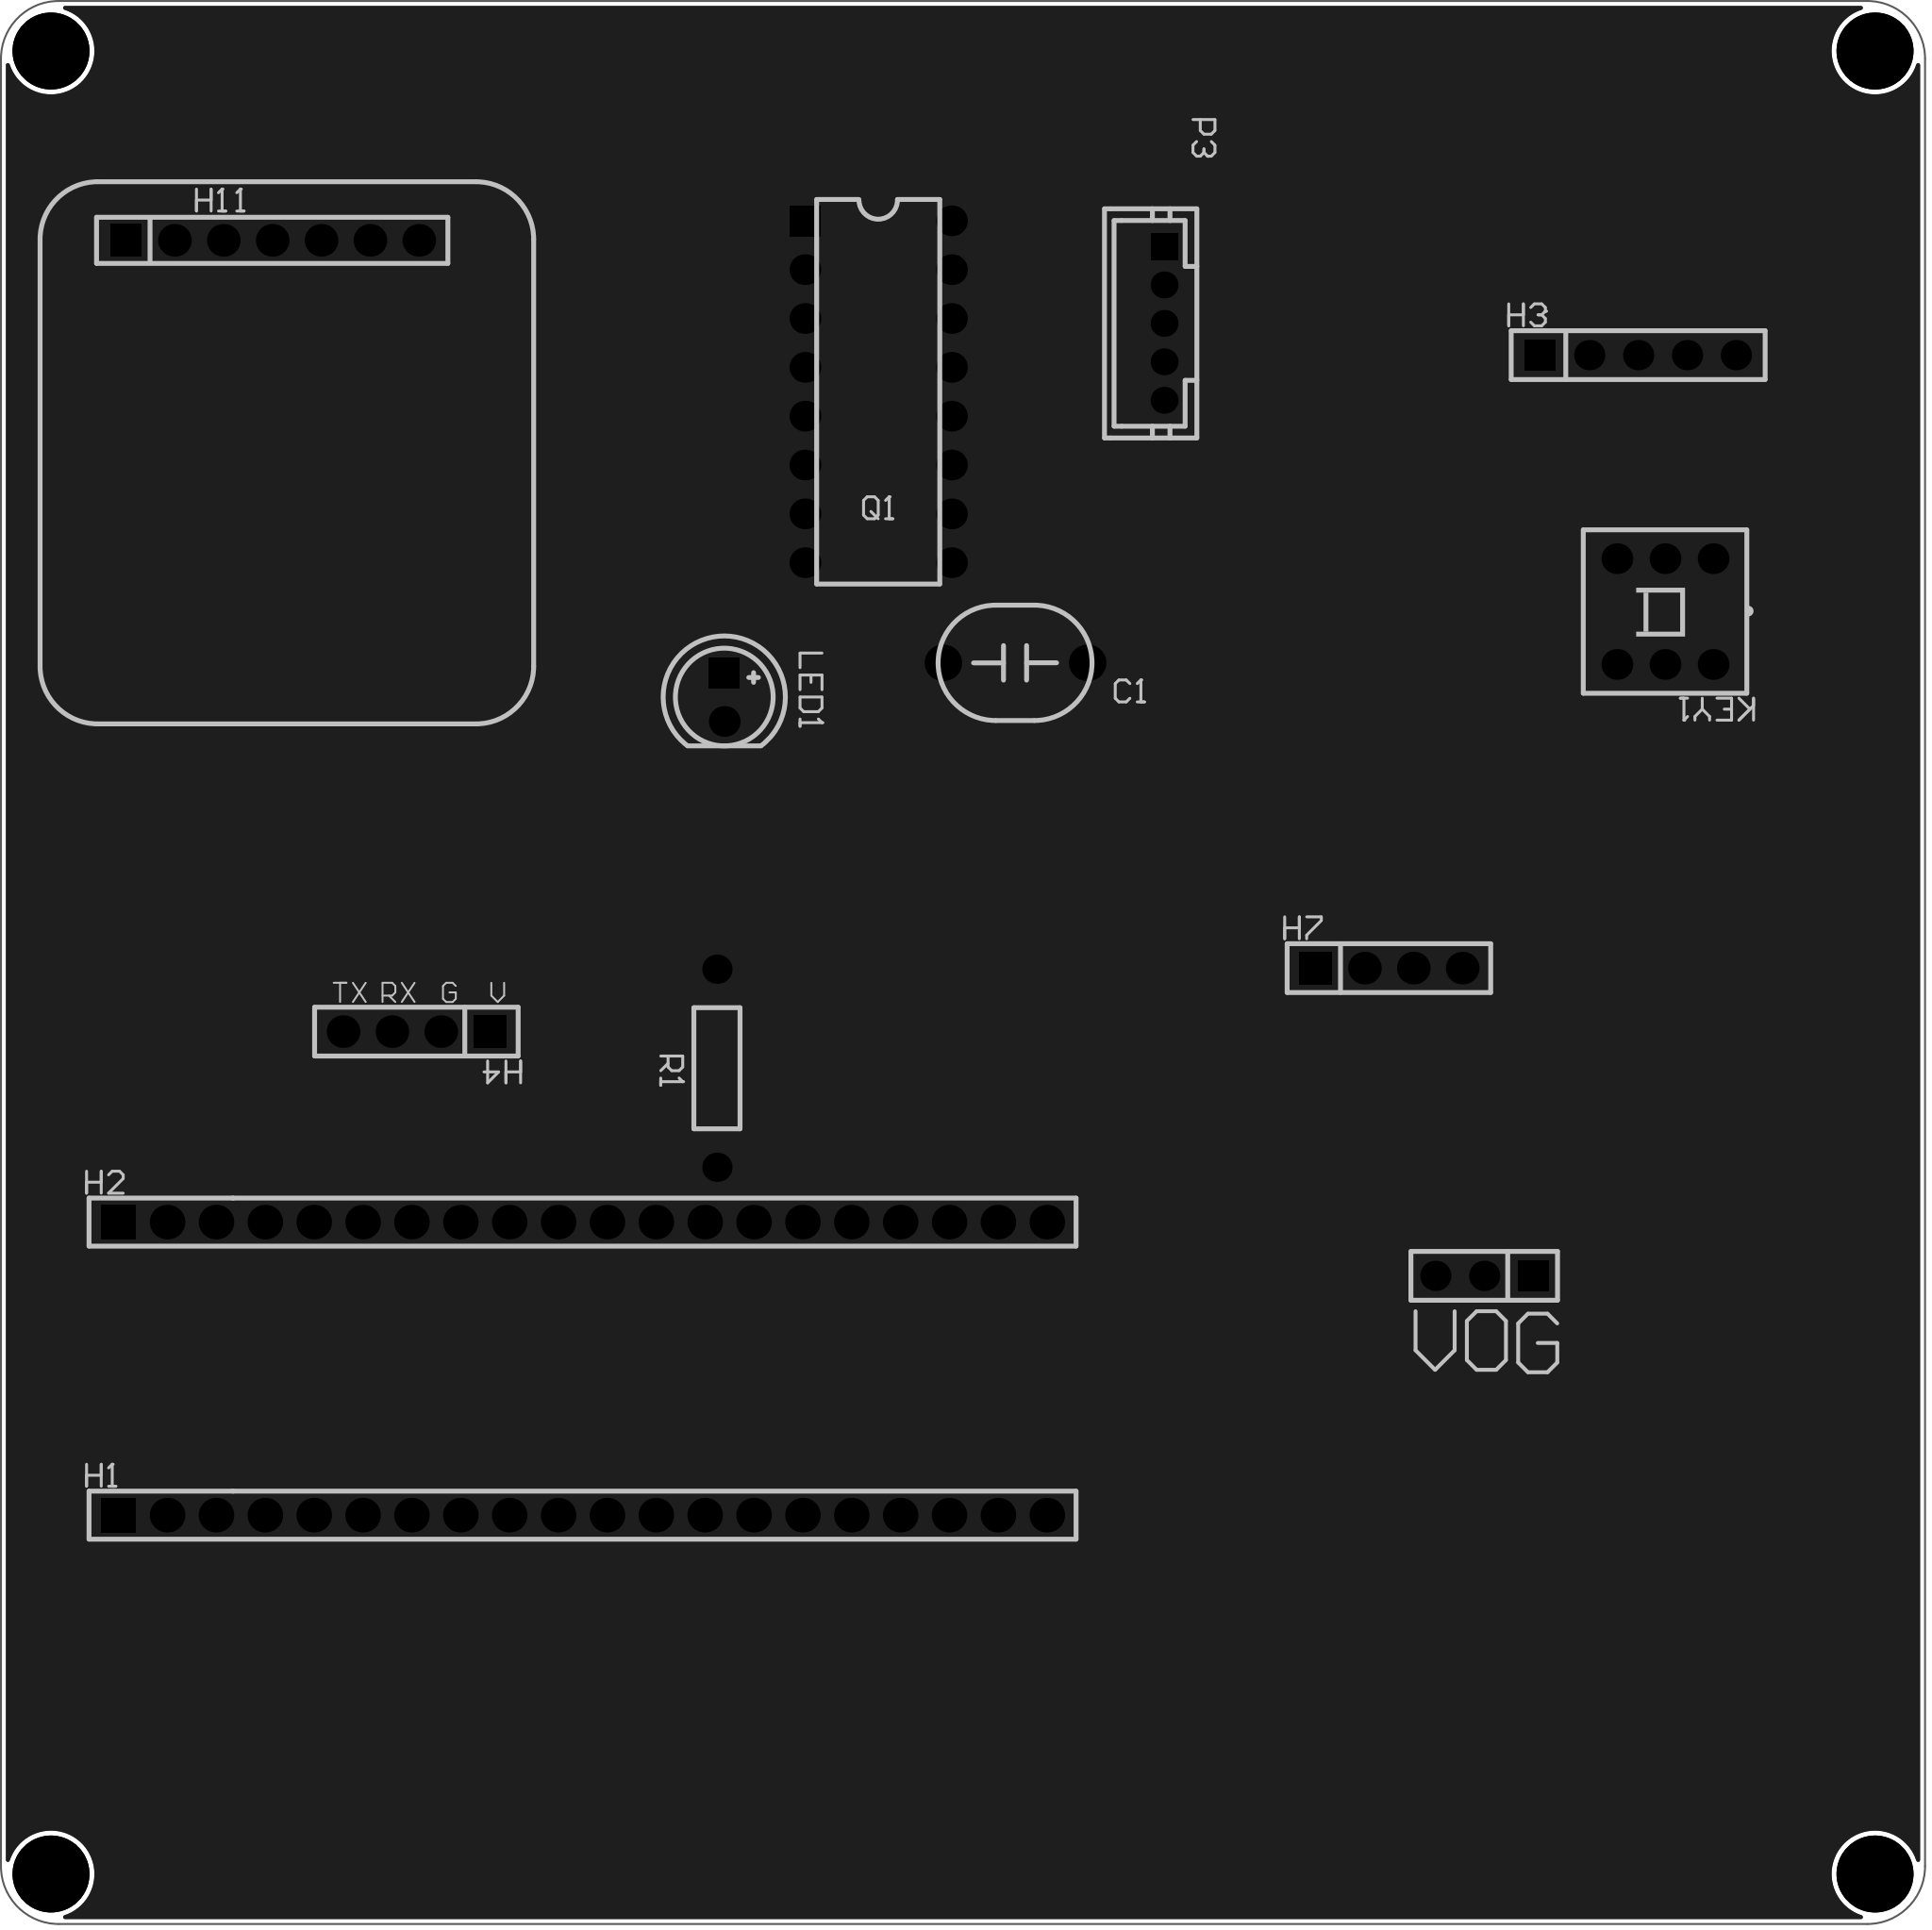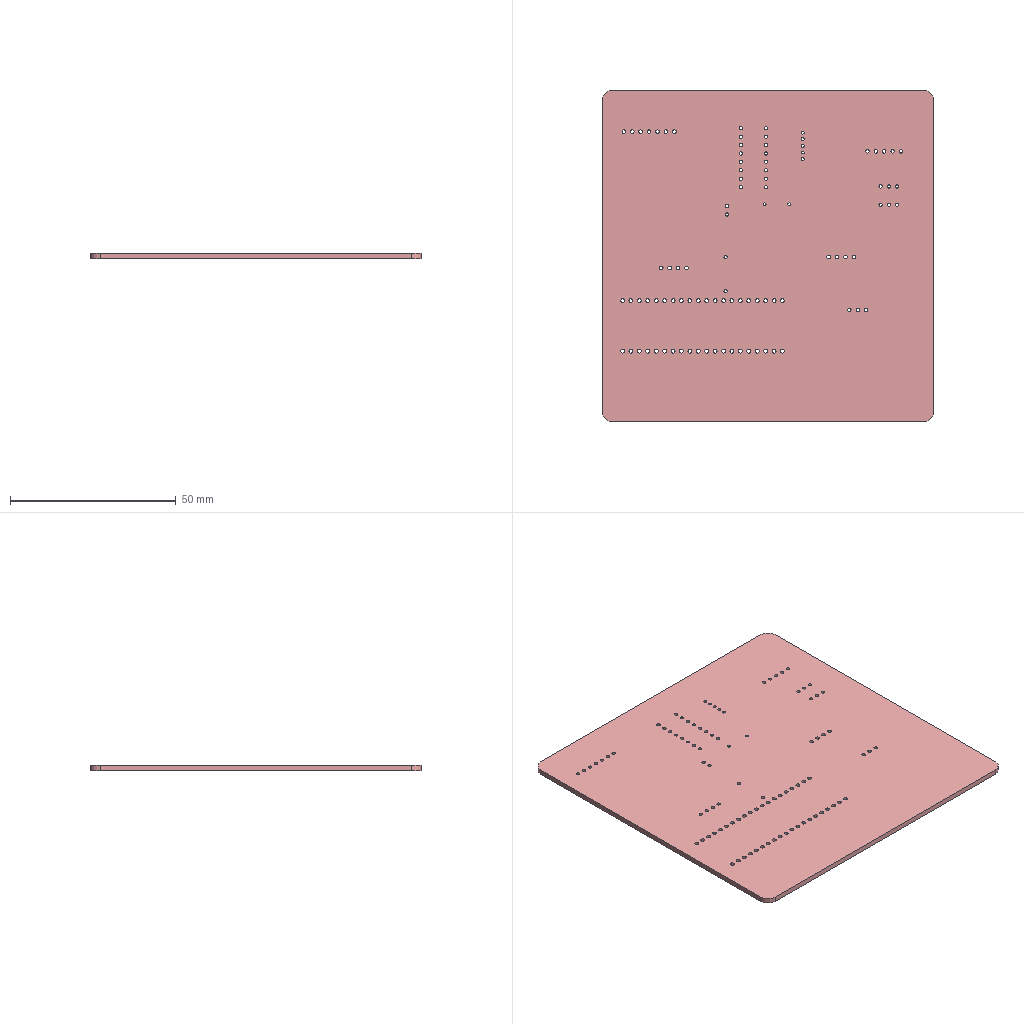Circuit board layout | Altium Designer | box 100 x 100 x 1.6 mm
Layer stack:
# Altium Designer layer stack of  (unit mm; dielectric type: 0 none, 1 core, 2 prepreg, 3 surface material)
index,name,kind,layer,copper_thickness_mm,dielectric_type,dielectric_thickness_mm,dielectric_material,dielectric_constant
0,Top Paste Mask Layer,other,,,,,,
1,Top Silkscreen Layer,other,,,,,,
2,Top Solder Mask Layer,dielectric,,,3,0.01,,3.3
3,Top Layer,copper,Top Layer,0.035,,,,
4,Dielectric1,dielectric,,,3,1.51,FR4,4.5
5,Bottom Layer,copper,Bottom Layer,0.035,,,,
6,Bottom Solder Mask Layer,dielectric,,,3,0.01,,3.3
7,Bottom Silkscreen Layer,other,,,,,,
8,Bottom Paste Mask Layer,other,,,,,,
# drill layer pairs: low layer,high layer
drill_pair,Top Layer,Bottom Layer
Part placement:
Designator,Comment,Layer,Footprint,Center-X(mm),Center-Y(mm),Rotation
H1,,TopLayer,HDR-TH_20P-P2.54-V-F,110.49,105.537,0
H2,,TopLayer,HDR-TH_20P-P2.54-V-F,110.49,120.777,0
H3,,TopLayer,HDR-TH_5P-P2.54-V-F,165.354,165.862,0
KEY1,Non-self-locking switch 8.5×8.5 silent,TopLayer,SW-TH_6P-L8.5-W8.5-P2.54,166.751,152.527,180
H4,,TopLayer,HDR-TH_4P-P2.54-V-F,101.854,130.683,180
H6,,TopLayer,HDR-TH_3P-P2.54-V-F,157.353,117.983,180
H7,,TopLayer,HDR-TH_4P-P2.54-V-F,152.4,133.985,0
H11,,TopLayer,HDR-TH_7P-P2.54-V-F,94.361,171.831,0
LED1,,TopLayer,LED_TH-_5mm,117.856,148.082,270
C1,10pF,TopLayer,CAP-TH_L5.5-W6.0-P7.50-D0.6,132.969,149.86,0
R1,1k,TopLayer,Res_1/4W,117.475,128.778,90
P3,PH2.0_5P through-hole socket,TopLayer,CONN-TH_5P-P2.00-PH5A,140.716,167.513,270
Q1,ULN2003,TopLayer,DIP-16_L19.8-W6.5-P2.54-LS7.6-BL,125.857,163.957,270
Pad and via stacks:
# Altium Designer via and pad stacks of  (unit mm). Each distinct definition once, with the count of objects using it.
# via: kind,start_layer,end_layer,hole_mm,diameter_mm,mode(0 simple;1 top-mid-bottom;2 full stack),diameter_per_layer,count,example_net
# pad: kind,layer,hole_mm,hole_type(0 round;1 square;2 slot),plating,top_size,top_shape(1 round;2 rect;3 octagon;9 rounded rect),mid_size,bottom_size,mode,footprint,size_per_layer,count,example
pad,Multi-Layer,1.2,0,plated,1.8x1.8,2,1.8x1.8,1.8x1.8,0,HDR-TH_20P-P2.54-V-F,,2,H1.1
pad,Multi-Layer,1.2,0,plated,1.8x1.8,1,1.8x1.8,1.8x1.8,0,HDR-TH_20P-P2.54-V-F,,38,H1.2
pad,Multi-Layer,1.02,0,plated,1.575x1.575,1,1.575x1.575,1.575x1.575,0,HDR-TH_5P-P2.54-V-F,,4,H3.5
pad,Multi-Layer,1.02,0,plated,1.575x1.575,2,1.575x1.575,1.575x1.575,0,HDR-TH_5P-P2.54-V-F,,1,H3.1
pad,Multi-Layer,1,0,plated,1.6x1.6,1,1.6x1.6,1.6x1.6,0,SW-TH_6P-L8.5-W8.5-P2.54,,6,KEY1.4
pad,Multi-Layer,1.1,0,plated,1.7x1.7,2,1.7x1.7,1.7x1.7,0,HDR-TH_4P-P2.54-V-F,,2,H4.1
pad,Multi-Layer,1.1,0,plated,1.7x1.7,1,1.7x1.7,1.7x1.7,0,HDR-TH_4P-P2.54-V-F,,6,H4.2
pad,Multi-Layer,1.02,0,plated,1.575x1.575,1,1.575x1.575,1.575x1.575,0,HDR-TH_3P-P2.54-V-F,,2,H6.3
pad,Multi-Layer,1.02,0,plated,1.575x1.575,2,1.575x1.575,1.575x1.575,0,HDR-TH_3P-P2.54-V-F,,1,H6.1
pad,Multi-Layer,1.1,0,plated,1.7x1.7,1,1.7x1.7,1.7x1.7,0,HDR-TH_7P-P2.54-V-F,,6,H11.7
pad,Multi-Layer,1.1,0,plated,1.575x1.7,2,1.575x1.7,1.575x1.7,0,HDR-TH_7P-P2.54-V-F,,1,H11.1
pad,Multi-Layer,1,0,plated,1.6x1.6,2,1.6x1.6,1.6x1.6,0,LED_TH-_5mm,,1,LED1.1
pad,Multi-Layer,1,0,plated,1.6x1.6,1,1.6x1.6,1.6x1.6,0,LED_TH-_5mm,,1,LED1.2
pad,Multi-Layer,0.9,0,plated,1.9x1.9,1,1.9x1.9,1.9x1.9,0,CAP-TH_L5.5-W6.0-P7.50-D0.6,,2,C1.1
pad,Multi-Layer,1,0,plated,1.524x1.524,1,1.524x1.524,1.524x1.524,0,Res_1/4W,,2,R1.1
pad,Multi-Layer,0.9,0,plated,1.4x1.4,2,1.4x1.4,1.4x1.4,0,CONN-TH_5P-P2.00-PH5A,,1,P3.1
pad,Multi-Layer,0.9,0,plated,1.4x1.4,1,1.4x1.4,1.4x1.4,0,CONN-TH_5P-P2.00-PH5A,,4,P3.2
pad,Multi-Layer,1,0,plated,1.6x1.6,1,1.6x1.6,1.6x1.6,0,DIP-16_L19.8-W6.5-P2.54-LS7.6-BL,,15,Q1.16
pad,Multi-Layer,1,0,plated,1.6x1.6,2,1.6x1.6,1.6x1.6,0,DIP-16_L19.8-W6.5-P2.54-LS7.6-BL,,1,Q1.1
via,Top Layer,Bottom Layer,3,4,0,,4,
Copper pours:
name,layer,net,type(0 solid;1 hatched;2 none)
Top Layer-GND,Top Layer,GND,0
Bottom Layer-GND,Bottom Layer,GND,0
Design rules, without the lines most boards share:
# Altium Designer design rules of  (exported by Altium Designer, unit mm)
# columns: name | kind | enabled | priority | scope1 | scope2 | descriptor | typed fields (field=value)
otherClearance | 52 | enabled | 1 | All | All | Hole To Hole Clearance (Gap=11.8mil) (All),(All) | gap=0.2997